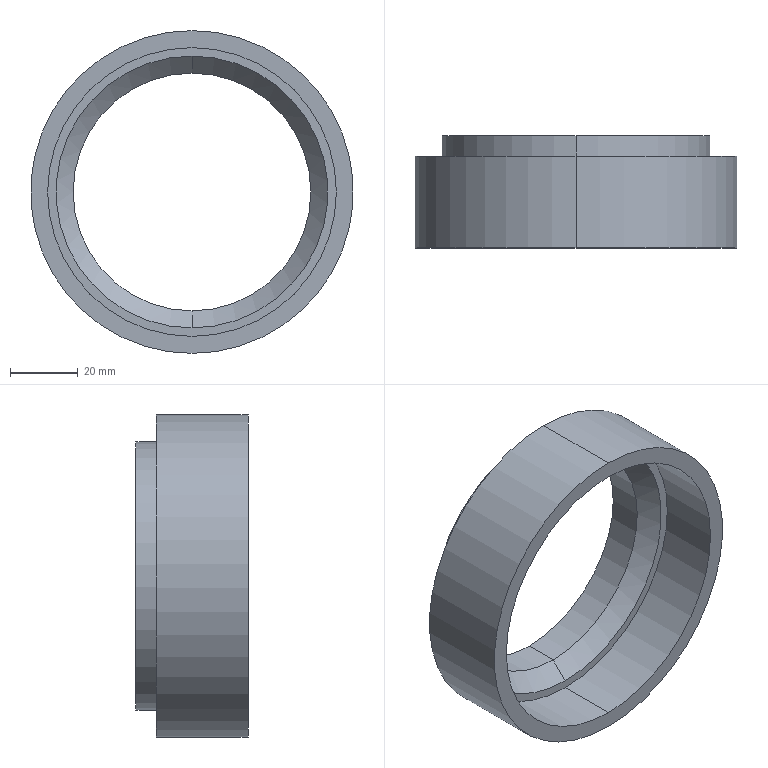Part | SolidWorks | features Chamfer 1, Revolution 1 | 1 solid | 14 faces | box 95 x 33 x 95 mm | volume 58044 mm3 | cylinder 8 | plane 4 | cone 2 | commonest cylinder face diameters 70 x2 79 x2 85 x2 95 x2
STEP:
#1=CARTESIAN_POINT('',(0.,23.,35.));
#2=VERTEX_POINT('',#1);
#3=CARTESIAN_POINT('',(0.,23.,-35.));
#4=VERTEX_POINT('',#3);
#5=CARTESIAN_POINT('',(0.,23.,0.));
#6=DIRECTION('',(0.,-1.,0.));
#7=DIRECTION('',(0.,0.,1.));
#8=AXIS2_PLACEMENT_3D('',#5,#6,#7);
#9=CIRCLE('',#8,35.);
#10=EDGE_CURVE('',#2,#4,#9,.T.);
#11=ORIENTED_EDGE('',*,*,#10,.F.);
#12=CARTESIAN_POINT('',(0.,18.,40.));
#13=VERTEX_POINT('',#12);
#14=CARTESIAN_POINT('',(0.,23.,35.));
#15=DIRECTION('',(0.,-0.7071,0.7071));
#16=VECTOR('',#15,1000.);
#17=LINE('',#14,#16);
#18=EDGE_CURVE('',#2,#13,#17,.T.);
#19=ORIENTED_EDGE('',*,*,#18,.T.);
#20=CARTESIAN_POINT('',(0.,18.,-40.));
#21=VERTEX_POINT('',#20);
#22=CARTESIAN_POINT('',(0.,18.,0.));
#23=DIRECTION('',(0.,1.,0.));
#24=DIRECTION('',(0.,0.,1.));
#25=AXIS2_PLACEMENT_3D('',#22,#23,#24);
#26=CIRCLE('',#25,40.);
#27=EDGE_CURVE('',#21,#13,#26,.T.);
#28=ORIENTED_EDGE('',*,*,#27,.F.);
#29=CARTESIAN_POINT('',(0.,23.,-35.));
#30=DIRECTION('',(0.,-0.7071,-0.7071));
#31=VECTOR('',#30,1000.);
#32=LINE('',#29,#31);
#33=EDGE_CURVE('',#4,#21,#32,.T.);
#34=ORIENTED_EDGE('',*,*,#33,.F.);
#35=EDGE_LOOP('',(#11,#19,#28,#34));
#36=FACE_OUTER_BOUND('',#35,.T.);
#37=CARTESIAN_POINT('',(0.,23.,0.));
#38=DIRECTION('',(0.,-1.,0.));
#39=DIRECTION('',(0.,0.,-1.));
#40=AXIS2_PLACEMENT_3D('',#37,#38,#39);
#41=CONICAL_SURFACE('',#40,35.,0.7854);
#42=ADVANCED_FACE('',(#36),#41,.F.);
#43=CARTESIAN_POINT('',(0.,18.,42.5));
#44=VERTEX_POINT('',#43);
#45=CARTESIAN_POINT('',(0.,18.,-42.5));
#46=VERTEX_POINT('',#45);
#47=CARTESIAN_POINT('',(0.,18.,0.));
#48=DIRECTION('',(0.,-1.,0.));
#49=DIRECTION('',(0.,0.,-1.));
#50=AXIS2_PLACEMENT_3D('',#47,#48,#49);
#51=CIRCLE('',#50,42.5);
#52=EDGE_CURVE('',#44,#46,#51,.T.);
#53=ORIENTED_EDGE('',*,*,#52,.F.);
#54=CARTESIAN_POINT('',(0.,0.,42.5));
#55=VERTEX_POINT('',#54);
#56=CARTESIAN_POINT('',(0.,0.,42.5));
#57=DIRECTION('',(0.,-1.,0.));
#58=VECTOR('',#57,1000.);
#59=LINE('',#56,#58);
#60=EDGE_CURVE('',#44,#55,#59,.T.);
#61=ORIENTED_EDGE('',*,*,#60,.T.);
#62=CARTESIAN_POINT('',(0.,0.,-42.5));
#63=VERTEX_POINT('',#62);
#64=CARTESIAN_POINT('',(0.,0.,0.));
#65=DIRECTION('',(0.,-1.,0.));
#66=DIRECTION('',(0.,0.,-1.));
#67=AXIS2_PLACEMENT_3D('',#64,#65,#66);
#68=CIRCLE('',#67,42.5);
#69=EDGE_CURVE('',#55,#63,#68,.T.);
#70=ORIENTED_EDGE('',*,*,#69,.T.);
#71=CARTESIAN_POINT('',(0.,0.,-42.5));
#72=DIRECTION('',(0.,-1.,0.));
#73=VECTOR('',#72,1000.);
#74=LINE('',#71,#73);
#75=EDGE_CURVE('',#46,#63,#74,.T.);
#76=ORIENTED_EDGE('',*,*,#75,.F.);
#77=EDGE_LOOP('',(#53,#61,#70,#76));
#78=FACE_OUTER_BOUND('',#77,.T.);
#79=CARTESIAN_POINT('',(0.,0.,0.));
#80=DIRECTION('',(0.,-1.,0.));
#81=DIRECTION('',(0.,0.,-1.));
#82=AXIS2_PLACEMENT_3D('',#79,#80,#81);
#83=CYLINDRICAL_SURFACE('',#82,42.5);
#84=ADVANCED_FACE('',(#78),#83,.F.);
#85=CARTESIAN_POINT('',(0.,27.,-47.5));
#86=VERTEX_POINT('',#85);
#87=CARTESIAN_POINT('',(0.,27.,47.5));
#88=VERTEX_POINT('',#87);
#89=CARTESIAN_POINT('',(0.,27.,0.));
#90=DIRECTION('',(0.,-1.,0.));
#91=DIRECTION('',(0.,0.,-1.));
#92=AXIS2_PLACEMENT_3D('',#89,#90,#91);
#93=CIRCLE('',#92,47.5);
#94=EDGE_CURVE('',#86,#88,#93,.T.);
#95=ORIENTED_EDGE('',*,*,#94,.T.);
#96=CARTESIAN_POINT('',(0.,0.,47.5));
#97=VERTEX_POINT('',#96);
#98=CARTESIAN_POINT('',(0.,0.,47.5));
#99=DIRECTION('',(0.,-1.,0.));
#100=VECTOR('',#99,1000.);
#101=LINE('',#98,#100);
#102=EDGE_CURVE('',#88,#97,#101,.T.);
#103=ORIENTED_EDGE('',*,*,#102,.T.);
#104=CARTESIAN_POINT('',(0.,0.,-47.5));
#105=VERTEX_POINT('',#104);
#106=CARTESIAN_POINT('',(0.,0.,0.));
#107=DIRECTION('',(0.,-1.,0.));
#108=DIRECTION('',(0.,0.,-1.));
#109=AXIS2_PLACEMENT_3D('',#106,#107,#108);
#110=CIRCLE('',#109,47.5);
#111=EDGE_CURVE('',#105,#97,#110,.T.);
#112=ORIENTED_EDGE('',*,*,#111,.F.);
#113=CARTESIAN_POINT('',(0.,0.,-47.5));
#114=DIRECTION('',(0.,-1.,0.));
#115=VECTOR('',#114,1000.);
#116=LINE('',#113,#115);
#117=EDGE_CURVE('',#86,#105,#116,.T.);
#118=ORIENTED_EDGE('',*,*,#117,.F.);
#119=EDGE_LOOP('',(#95,#103,#112,#118));
#120=FACE_OUTER_BOUND('',#119,.T.);
#121=CARTESIAN_POINT('',(0.,0.,0.));
#122=DIRECTION('',(0.,-1.,0.));
#123=DIRECTION('',(0.,0.,-1.));
#124=AXIS2_PLACEMENT_3D('',#121,#122,#123);
#125=CYLINDRICAL_SURFACE('',#124,47.5);
#126=ADVANCED_FACE('',(#120),#125,.T.);
#127=CARTESIAN_POINT('',(0.,33.,-39.5));
#128=VERTEX_POINT('',#127);
#129=CARTESIAN_POINT('',(0.,33.,39.5));
#130=VERTEX_POINT('',#129);
#131=CARTESIAN_POINT('',(0.,33.,0.));
#132=DIRECTION('',(0.,-1.,0.));
#133=DIRECTION('',(0.,0.,-1.));
#134=AXIS2_PLACEMENT_3D('',#131,#132,#133);
#135=CIRCLE('',#134,39.5);
#136=EDGE_CURVE('',#128,#130,#135,.T.);
#137=ORIENTED_EDGE('',*,*,#136,.T.);
#138=CARTESIAN_POINT('',(0.,27.,39.5));
#139=VERTEX_POINT('',#138);
#140=CARTESIAN_POINT('',(0.,0.,39.5));
#141=DIRECTION('',(0.,-1.,0.));
#142=VECTOR('',#141,1000.);
#143=LINE('',#140,#142);
#144=EDGE_CURVE('',#130,#139,#143,.T.);
#145=ORIENTED_EDGE('',*,*,#144,.T.);
#146=CARTESIAN_POINT('',(0.,27.,-39.5));
#147=VERTEX_POINT('',#146);
#148=CARTESIAN_POINT('',(0.,27.,0.));
#149=DIRECTION('',(0.,-1.,0.));
#150=DIRECTION('',(0.,0.,-1.));
#151=AXIS2_PLACEMENT_3D('',#148,#149,#150);
#152=CIRCLE('',#151,39.5);
#153=EDGE_CURVE('',#147,#139,#152,.T.);
#154=ORIENTED_EDGE('',*,*,#153,.F.);
#155=CARTESIAN_POINT('',(0.,0.,-39.5));
#156=DIRECTION('',(0.,-1.,0.));
#157=VECTOR('',#156,1000.);
#158=LINE('',#155,#157);
#159=EDGE_CURVE('',#128,#147,#158,.T.);
#160=ORIENTED_EDGE('',*,*,#159,.F.);
#161=EDGE_LOOP('',(#137,#145,#154,#160));
#162=FACE_OUTER_BOUND('',#161,.T.);
#163=CARTESIAN_POINT('',(0.,0.,0.));
#164=DIRECTION('',(0.,-1.,0.));
#165=DIRECTION('',(0.,0.,-1.));
#166=AXIS2_PLACEMENT_3D('',#163,#164,#165);
#167=CYLINDRICAL_SURFACE('',#166,39.5);
#168=ADVANCED_FACE('',(#162),#167,.T.);
#169=CARTESIAN_POINT('',(0.,33.,35.));
#170=VERTEX_POINT('',#169);
#171=CARTESIAN_POINT('',(0.,33.,-35.));
#172=VERTEX_POINT('',#171);
#173=CARTESIAN_POINT('',(0.,33.,0.));
#174=DIRECTION('',(0.,-1.,0.));
#175=DIRECTION('',(0.,0.,-1.));
#176=AXIS2_PLACEMENT_3D('',#173,#174,#175);
#177=CIRCLE('',#176,35.);
#178=EDGE_CURVE('',#170,#172,#177,.T.);
#179=ORIENTED_EDGE('',*,*,#178,.F.);
#180=CARTESIAN_POINT('',(0.,0.,35.));
#181=DIRECTION('',(0.,-1.,0.));
#182=VECTOR('',#181,1000.);
#183=LINE('',#180,#182);
#184=EDGE_CURVE('',#170,#2,#183,.T.);
#185=ORIENTED_EDGE('',*,*,#184,.T.);
#186=ORIENTED_EDGE('',*,*,#10,.T.);
#187=CARTESIAN_POINT('',(0.,0.,-35.));
#188=DIRECTION('',(0.,-1.,0.));
#189=VECTOR('',#188,1000.);
#190=LINE('',#187,#189);
#191=EDGE_CURVE('',#172,#4,#190,.T.);
#192=ORIENTED_EDGE('',*,*,#191,.F.);
#193=EDGE_LOOP('',(#179,#185,#186,#192));
#194=FACE_OUTER_BOUND('',#193,.T.);
#195=CARTESIAN_POINT('',(0.,0.,0.));
#196=DIRECTION('',(0.,-1.,0.));
#197=DIRECTION('',(0.,0.,-1.));
#198=AXIS2_PLACEMENT_3D('',#195,#196,#197);
#199=CYLINDRICAL_SURFACE('',#198,35.);
#200=ADVANCED_FACE('',(#194),#199,.F.);
#201=ORIENTED_EDGE('',*,*,#184,.F.);
#202=CARTESIAN_POINT('',(0.,33.,0.));
#203=DIRECTION('',(0.,-1.,0.));
#204=DIRECTION('',(0.,0.,-1.));
#205=AXIS2_PLACEMENT_3D('',#202,#203,#204);
#206=CIRCLE('',#205,35.);
#207=EDGE_CURVE('',#172,#170,#206,.T.);
#208=ORIENTED_EDGE('',*,*,#207,.F.);
#209=ORIENTED_EDGE('',*,*,#191,.T.);
#210=CARTESIAN_POINT('',(0.,23.,0.));
#211=DIRECTION('',(0.,-1.,0.));
#212=DIRECTION('',(0.,0.,1.));
#213=AXIS2_PLACEMENT_3D('',#210,#211,#212);
#214=CIRCLE('',#213,35.);
#215=EDGE_CURVE('',#4,#2,#214,.T.);
#216=ORIENTED_EDGE('',*,*,#215,.T.);
#217=EDGE_LOOP('',(#201,#208,#209,#216));
#218=FACE_OUTER_BOUND('',#217,.T.);
#219=CARTESIAN_POINT('',(0.,0.,0.));
#220=DIRECTION('',(0.,-1.,0.));
#221=DIRECTION('',(0.,0.,-1.));
#222=AXIS2_PLACEMENT_3D('',#219,#220,#221);
#223=CYLINDRICAL_SURFACE('',#222,35.);
#224=ADVANCED_FACE('',(#218),#223,.F.);
#225=ORIENTED_EDGE('',*,*,#136,.F.);
#226=CARTESIAN_POINT('',(0.,33.,0.));
#227=DIRECTION('',(0.,-1.,0.));
#228=DIRECTION('',(0.,0.,-1.));
#229=AXIS2_PLACEMENT_3D('',#226,#227,#228);
#230=CIRCLE('',#229,39.5);
#231=EDGE_CURVE('',#130,#128,#230,.T.);
#232=ORIENTED_EDGE('',*,*,#231,.F.);
#233=EDGE_LOOP('',(#225,#232));
#234=FACE_OUTER_BOUND('',#233,.T.);
#235=ORIENTED_EDGE('',*,*,#207,.T.);
#236=ORIENTED_EDGE('',*,*,#178,.T.);
#237=EDGE_LOOP('',(#235,#236));
#238=FACE_BOUND('',#237,.T.);
#239=CARTESIAN_POINT('',(-35.,33.,0.));
#240=DIRECTION('',(0.,-1.,0.));
#241=DIRECTION('',(0.,0.,-1.));
#242=AXIS2_PLACEMENT_3D('',#239,#240,#241);
#243=PLANE('',#242);
#244=ADVANCED_FACE('',(#234,#238),#243,.F.);
#245=ORIENTED_EDGE('',*,*,#144,.F.);
#246=ORIENTED_EDGE('',*,*,#231,.T.);
#247=ORIENTED_EDGE('',*,*,#159,.T.);
#248=CARTESIAN_POINT('',(0.,27.,0.));
#249=DIRECTION('',(0.,-1.,0.));
#250=DIRECTION('',(0.,0.,-1.));
#251=AXIS2_PLACEMENT_3D('',#248,#249,#250);
#252=CIRCLE('',#251,39.5);
#253=EDGE_CURVE('',#139,#147,#252,.T.);
#254=ORIENTED_EDGE('',*,*,#253,.F.);
#255=EDGE_LOOP('',(#245,#246,#247,#254));
#256=FACE_OUTER_BOUND('',#255,.T.);
#257=CARTESIAN_POINT('',(0.,0.,0.));
#258=DIRECTION('',(0.,-1.,0.));
#259=DIRECTION('',(0.,0.,-1.));
#260=AXIS2_PLACEMENT_3D('',#257,#258,#259);
#261=CYLINDRICAL_SURFACE('',#260,39.5);
#262=ADVANCED_FACE('',(#256),#261,.T.);
#263=ORIENTED_EDGE('',*,*,#94,.F.);
#264=CARTESIAN_POINT('',(0.,27.,0.));
#265=DIRECTION('',(0.,-1.,0.));
#266=DIRECTION('',(0.,0.,-1.));
#267=AXIS2_PLACEMENT_3D('',#264,#265,#266);
#268=CIRCLE('',#267,47.5);
#269=EDGE_CURVE('',#88,#86,#268,.T.);
#270=ORIENTED_EDGE('',*,*,#269,.F.);
#271=EDGE_LOOP('',(#263,#270));
#272=FACE_OUTER_BOUND('',#271,.T.);
#273=ORIENTED_EDGE('',*,*,#153,.T.);
#274=ORIENTED_EDGE('',*,*,#253,.T.);
#275=EDGE_LOOP('',(#273,#274));
#276=FACE_BOUND('',#275,.T.);
#277=CARTESIAN_POINT('',(-39.5,27.,0.));
#278=DIRECTION('',(0.,-1.,0.));
#279=DIRECTION('',(0.,0.,-1.));
#280=AXIS2_PLACEMENT_3D('',#277,#278,#279);
#281=PLANE('',#280);
#282=ADVANCED_FACE('',(#272,#276),#281,.F.);
#283=ORIENTED_EDGE('',*,*,#102,.F.);
#284=ORIENTED_EDGE('',*,*,#269,.T.);
#285=ORIENTED_EDGE('',*,*,#117,.T.);
#286=CARTESIAN_POINT('',(0.,0.,0.));
#287=DIRECTION('',(0.,-1.,0.));
#288=DIRECTION('',(0.,0.,-1.));
#289=AXIS2_PLACEMENT_3D('',#286,#287,#288);
#290=CIRCLE('',#289,47.5);
#291=EDGE_CURVE('',#97,#105,#290,.T.);
#292=ORIENTED_EDGE('',*,*,#291,.F.);
#293=EDGE_LOOP('',(#283,#284,#285,#292));
#294=FACE_OUTER_BOUND('',#293,.T.);
#295=CARTESIAN_POINT('',(0.,0.,0.));
#296=DIRECTION('',(0.,-1.,0.));
#297=DIRECTION('',(0.,0.,-1.));
#298=AXIS2_PLACEMENT_3D('',#295,#296,#297);
#299=CYLINDRICAL_SURFACE('',#298,47.5);
#300=ADVANCED_FACE('',(#294),#299,.T.);
#301=CARTESIAN_POINT('',(0.,0.,0.));
#302=DIRECTION('',(0.,-1.,0.));
#303=DIRECTION('',(0.,0.,-1.));
#304=AXIS2_PLACEMENT_3D('',#301,#302,#303);
#305=CIRCLE('',#304,42.5);
#306=EDGE_CURVE('',#63,#55,#305,.T.);
#307=ORIENTED_EDGE('',*,*,#306,.F.);
#308=ORIENTED_EDGE('',*,*,#69,.F.);
#309=EDGE_LOOP('',(#307,#308));
#310=FACE_BOUND('',#309,.T.);
#311=ORIENTED_EDGE('',*,*,#111,.T.);
#312=ORIENTED_EDGE('',*,*,#291,.T.);
#313=EDGE_LOOP('',(#311,#312));
#314=FACE_OUTER_BOUND('',#313,.T.);
#315=CARTESIAN_POINT('',(-47.5,0.,0.));
#316=DIRECTION('',(0.,1.,0.));
#317=DIRECTION('',(0.,0.,1.));
#318=AXIS2_PLACEMENT_3D('',#315,#316,#317);
#319=PLANE('',#318);
#320=ADVANCED_FACE('',(#310,#314),#319,.F.);
#321=ORIENTED_EDGE('',*,*,#60,.F.);
#322=CARTESIAN_POINT('',(0.,18.,0.));
#323=DIRECTION('',(0.,-1.,0.));
#324=DIRECTION('',(0.,0.,-1.));
#325=AXIS2_PLACEMENT_3D('',#322,#323,#324);
#326=CIRCLE('',#325,42.5);
#327=EDGE_CURVE('',#46,#44,#326,.T.);
#328=ORIENTED_EDGE('',*,*,#327,.F.);
#329=ORIENTED_EDGE('',*,*,#75,.T.);
#330=ORIENTED_EDGE('',*,*,#306,.T.);
#331=EDGE_LOOP('',(#321,#328,#329,#330));
#332=FACE_OUTER_BOUND('',#331,.T.);
#333=CARTESIAN_POINT('',(0.,0.,0.));
#334=DIRECTION('',(0.,-1.,0.));
#335=DIRECTION('',(0.,0.,-1.));
#336=AXIS2_PLACEMENT_3D('',#333,#334,#335);
#337=CYLINDRICAL_SURFACE('',#336,42.5);
#338=ADVANCED_FACE('',(#332),#337,.F.);
#339=ORIENTED_EDGE('',*,*,#27,.T.);
#340=CARTESIAN_POINT('',(0.,18.,0.));
#341=DIRECTION('',(0.,1.,0.));
#342=DIRECTION('',(0.,0.,1.));
#343=AXIS2_PLACEMENT_3D('',#340,#341,#342);
#344=CIRCLE('',#343,40.);
#345=EDGE_CURVE('',#13,#21,#344,.T.);
#346=ORIENTED_EDGE('',*,*,#345,.T.);
#347=EDGE_LOOP('',(#339,#346));
#348=FACE_BOUND('',#347,.T.);
#349=ORIENTED_EDGE('',*,*,#327,.T.);
#350=ORIENTED_EDGE('',*,*,#52,.T.);
#351=EDGE_LOOP('',(#349,#350));
#352=FACE_OUTER_BOUND('',#351,.T.);
#353=CARTESIAN_POINT('',(-42.5,18.,0.));
#354=DIRECTION('',(0.,1.,0.));
#355=DIRECTION('',(0.,0.,1.));
#356=AXIS2_PLACEMENT_3D('',#353,#354,#355);
#357=PLANE('',#356);
#358=ADVANCED_FACE('',(#348,#352),#357,.F.);
#359=ORIENTED_EDGE('',*,*,#18,.F.);
#360=ORIENTED_EDGE('',*,*,#215,.F.);
#361=ORIENTED_EDGE('',*,*,#33,.T.);
#362=ORIENTED_EDGE('',*,*,#345,.F.);
#363=EDGE_LOOP('',(#359,#360,#361,#362));
#364=FACE_OUTER_BOUND('',#363,.T.);
#365=CARTESIAN_POINT('',(0.,23.,0.));
#366=DIRECTION('',(0.,-1.,0.));
#367=DIRECTION('',(0.,0.,-1.));
#368=AXIS2_PLACEMENT_3D('',#365,#366,#367);
#369=CONICAL_SURFACE('',#368,35.,0.7854);
#370=ADVANCED_FACE('',(#364),#369,.F.);
#371=CLOSED_SHELL('',(#42,#84,#126,#168,#200,#224,#244,#262,#282,#300,#320,#338,#358,#370));
#372=MANIFOLD_SOLID_BREP('',#371);
#373=CARTESIAN_POINT('',(0.,0.,0.));
#374=DIRECTION('',(0.,0.,1.));
#375=DIRECTION('',(1.,0.,0.));
#376=AXIS2_PLACEMENT_3D('',#373,#374,#375);
#377=(LENGTH_UNIT()NAMED_UNIT(*)SI_UNIT(.MILLI.,.METRE.));
#378=UNCERTAINTY_MEASURE_WITH_UNIT(LENGTH_MEASURE(0.00001),#377,'','');
#379=(NAMED_UNIT(*)PLANE_ANGLE_UNIT()SI_UNIT($,.RADIAN.));
#380=(NAMED_UNIT(*)SI_UNIT($,.STERADIAN.)SOLID_ANGLE_UNIT());
#381=(GEOMETRIC_REPRESENTATION_CONTEXT(3)GLOBAL_UNCERTAINTY_ASSIGNED_CONTEXT((#378))GLOBAL_UNIT_ASSIGNED_CONTEXT((#377,#379,#380))REPRESENTATION_CONTEXT('',''));
#382=ADVANCED_BREP_SHAPE_REPRESENTATION('',(#372,#376),#381);